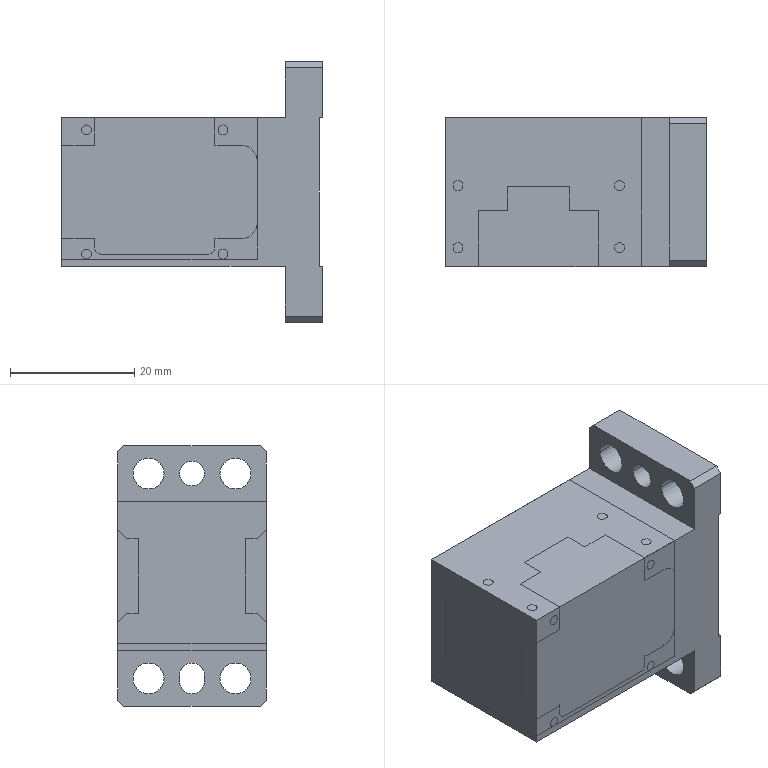CAM job | NX | 3+2 milling, drilling | part box 42 x 24 x 42 mm
Tools:
number,name,description,diameter,corner_radius,flute_length,length,flutes
1,D63,Milling Tool-5 Parameters,63.0,0.0,50.0,75.0,2
11,D10JING,Milling Tool-5 Parameters,10.0,0.0,50.0,75.0,2
10,D10,Milling Tool-5 Parameters,10.0,0.0,50.0,75.0,2
4,D4,Milling Tool-5 Parameters,4.0,0.0,50.0,75.0,2
7,D6A45,Milling Tool-5 Parameters,6.0,0.0,50.0,75.0,2
16,1.6ZT,Drilling Tool,1.6,0.0,35.0,50.0,2
14,5.0ZT,Drilling Tool,4.5,0.0,35.0,50.0,2
3,D3,Milling Tool-5 Parameters,3.0,0.0,50.0,75.0,2
6,D6,Milling Tool-5 Parameters,6.0,0.0,50.0,75.0,2
2,D2,Milling Tool-5 Parameters,2.0,0.0,50.0,75.0,2
9,D3ZXZ,Milling Tool-5 Parameters,3.0,0.0,50.0,75.0,2
5,D4R0.5,Milling Tool-5 Parameters,4.0,0.5,50.0,75.0,2
8,ZXZ,Milling Tool-5 Parameters,6.0,0.0,50.0,75.0,2
15,D6JING,Milling Tool-5 Parameters,6.0,0.0,50.0,75.0,2
Operations:
program,operation,operation_type,tool,method,geometry_group,spindle_rpm,surface_speed,feed_per_tooth,feed_cut,feed_plunge,cut_length_mm,path_length_mm,cut_time_min,machine_time_min
1,FLOOR_WALL,VolumeBased25DMillingOperation,D63,METHOD,A,2000.0,395.0,0.3,1200.0,100.0,121.0,175.0,0.1008,0.1062
1,ZLEVEL_PROFILE,ZLevelMilling,D10,METHOD,A,3000.0,94.0,0.3,1800.0,1000.0,46138.369,46237.369,25.646,25.656
1,FLOOR_WALL_1,VolumeBased25DMillingOperation,D10,METHOD,A,3000.0,94.0,0.3083,1850.0,1000.0,13885.356,14943.977,7.767,7.873
1,CAVITY_MILL_COPY_1,CavityMilling,D10JING,METHOD,A,5000.0,157.0,0.1,1000.0,1000.0,512.263,778.982,0.5123,0.5389
1,FLOOR_WALL_1_1,VolumeBased25DMillingOperation,D10JING,METHOD,A,5500.0,172.0,0.1136,1250.0,100.0,355.76,506.26,0.2846,0.2997
1,PLANAR_MILL,PlanarMilling,D6A45,METHOD,A,7500.0,141.0,0.0833,1250.0,100.0,98.339,175.339,0.0787,0.0864
1,PLANAR_MILL_COPY,PlanarMilling,D6A45,METHOD,A,7500.0,141.0,0.0833,1250.0,100.0,74.477,135.477,0.0596,0.0657
2,FLOOR_WALL_COPY,VolumeBased25DMillingOperation,D63,METHOD,B,2000.0,395.0,0.25,1000.0,100.0,1755.0,4077.004,1.755,1.987
2,FLOOR_WALL_1_COPY,VolumeBased25DMillingOperation,D10,METHOD,B,3000.0,94.0,0.3333,2000.0,1000.0,13885.356,14943.977,7.227,7.333
2,FLOOR_WALL_1_1_COPY,VolumeBased25DMillingOperation,D10JING,METHOD,B,5500.0,172.0,0.1136,1250.0,100.0,355.76,506.26,0.2846,0.2997
2,DRILLING,Operation,D6A45,METHOD,B,5000.0,94.0,0.025,250.0,0.0,16.4,200.163,0.0656,0.084
2,DRILLING_COPY,Operation,1.6ZT,METHOD,B,2000.0,10.0,0.025,100.0,0.0,33.923,235.208,0.3392,0.3594
2,PLANAR_MILL_COPY_1,PlanarMilling,D6A45,METHOD,B,7500.0,141.0,0.0833,1250.0,100.0,98.339,175.339,0.0787,0.0864
2,PLANAR_MILL_COPY_COPY,PlanarMilling,D6A45,METHOD,B,7500.0,141.0,0.0833,1250.0,100.0,74.477,135.477,0.0596,0.0657
3,FLOOR_WALL_1_COPY_1,VolumeBased25DMillingOperation,D10JING,METHOD,C,5500.0,172.0,0.1364,1500.0,1000.0,387.068,469.068,0.2675,0.2757
3,DRILLING_1,Operation,ZXZ,METHOD,C,5000.0,94.0,0.025,250.0,0.0,20.0,174.685,0.08,0.0955
3,DRILLING_COPY_1,Operation,5.0ZT,METHOD,C,2000.0,28.0,0.05,200.0,0.0,47.408,225.587,0.237,0.2549
3,ZLEVEL_PROFILE_1,ZLevelMilling,D3,METHOD,C,6000.0,56.0,0.0833,1000.0,100.0,1557.647,1718.14,1.558,1.574
3,PLANAR_MILL_COPY_2,PlanarMilling,D6A45,METHOD,C,7500.0,141.0,0.0833,1250.0,100.0,197.088,750.739,0.1577,0.213
3,PLANAR_MILL_COPY_2_COPY,PlanarMilling,D6A45,METHOD,C,7500.0,141.0,0.0833,1250.0,100.0,53.295,202.033,0.0426,0.0575
3,刀补,ZLevelMilling,D3,METHOD,C,6500.0,61.0,0.0769,1000.0,100.0,22.279,88.279,0.0223,0.0289
3,刀补3,CylinderMilling,D3,METHOD,C,6500.0,61.0,0.0769,1000.0,100.0,15.482,80.982,0.0155,0.022
4,CAVITY_MILL,CavityMilling,D6,METHOD,D,4500.0,84.0,0.2222,2000.0,1000.0,34163.154,37401.673,18.899,19.223
4,FLOOR_WALL_1_1_COPY_1,VolumeBased25DMillingOperation,D6JING,METHOD,D,7500.0,141.0,0.0767,1150.0,100.0,436.716,1683.133,0.3798,0.5044
4,CAVITY_MILL_COPY_1_COPY,CavityMilling,D6JING,METHOD,D,7500.0,141.0,0.0667,1000.0,1000.0,173.133,319.331,0.1731,0.1878
4,CAVITY_MILL_COPY,CavityMilling,D2,METHOD,D,6500.0,40.0,0.0615,800.0,1000.0,21029.434,32457.893,25.265,26.408
4,DRILLING_1_COPY,Operation,D3ZXZ,METHOD,D,5000.0,94.0,0.025,250.0,0.0,32.8,237.678,0.1312,0.1517
4,DRILLING_COPY_COPY,Operation,1.6ZT,METHOD,D,2000.0,10.0,0.025,100.0,0.0,69.445,310.969,0.6945,0.7186
4,ZLEVEL_PROFILE_2,ZLevelMilling,D4R0.5,METHOD,D,7500.0,94.0,0.2,3000.0,100.0,897.946,1173.843,0.2993,0.3269
4,PLANAR_MILL_COPY_2_COPY_1,PlanarMilling,D6A45,METHOD,D,7500.0,141.0,0.0833,1250.0,100.0,49.847,251.766,0.0399,0.0601
4,刀补6,CavityMilling,D6JING,METHOD,D,7500.0,141.0,0.0667,1000.0,1000.0,173.733,319.762,0.1737,0.1883
4,刀补66,CavityMilling,D6JING,METHOD,D,7500.0,141.0,0.0667,1000.0,1000.0,65.545,130.405,0.0655,0.072
5,DRILLING_COPY_2,Operation,ZXZ,METHOD,E,5000.0,94.0,0.025,250.0,0.0,16.4,164.451,0.0656,0.0804
5,DRILLING_COPY_COPY_1,Operation,1.6ZT,METHOD,E,2000.0,10.0,0.025,100.0,0.0,34.723,201.097,0.3472,0.3639
5,FLOOR_WALL_1_COPY_COPY,VolumeBased25DMillingOperation,D6,METHOD,E,4500.0,84.0,0.2222,2000.0,1000.0,2275.179,2573.806,1.251,1.281
5,ZLEVEL_PROFILE_2_COPY,ZLevelMilling,D4R0.5,METHOD,E,6500.0,81.0,0.2308,3000.0,100.0,1949.714,2084.942,0.6499,0.6634
5,CAVITY_MILL_COPY_COPY,CavityMilling,D2,METHOD,E,5500.0,34.0,0.0727,800.0,1000.0,674.669,1114.641,0.8095,0.8535
5,刀补4,PlanarMilling,D4,METHOD,E,6500.0,81.0,0.0769,1000.0,100.0,68.987,133.687,0.069,0.0755